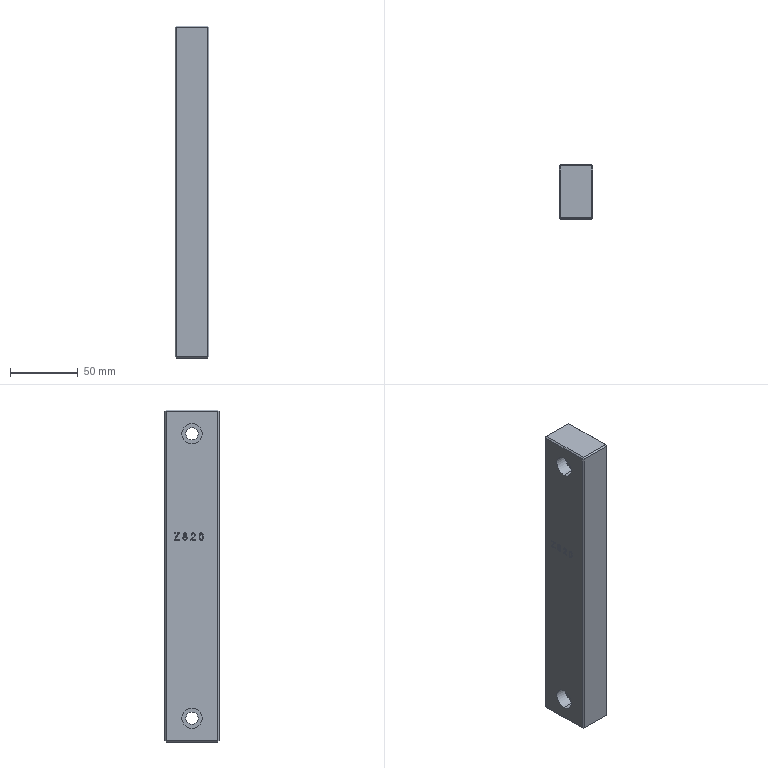Part | Creo | 1 solid | 130 faces | box 25 x 40 x 245 mm | volume 239163 mm3 | other 73 | plane 46 | cylinder 11 | commonest cylinder face diameters 9 x4 15 x4 2.686 x1 4.658 x1 73.459 x1